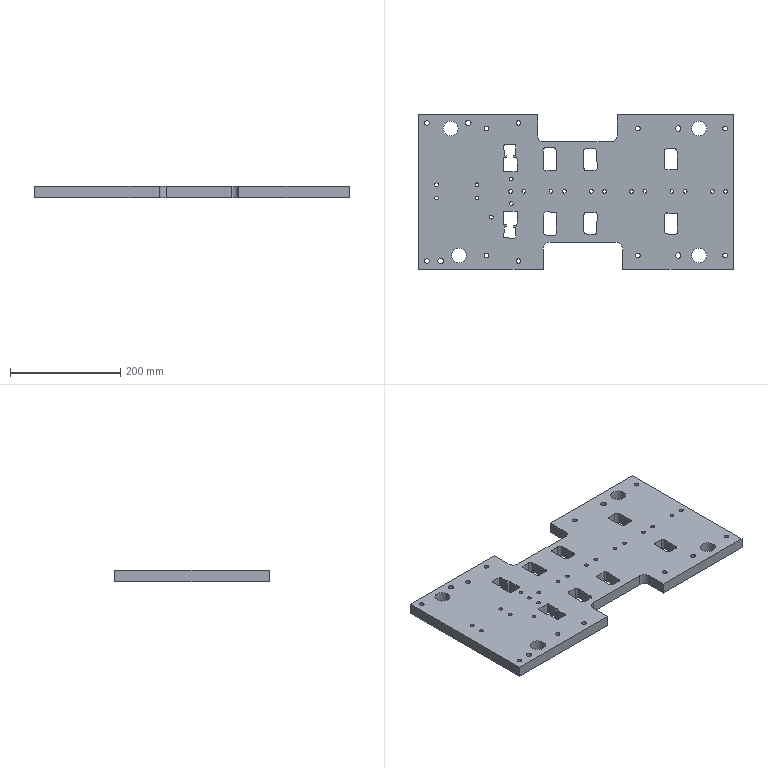Part | NX | features PPS-2 2 | 1 solid | 169 faces | box 570 x 280 x 20 mm | volume 2679314 mm3 | cylinder 94 | plane 62 | cone 13 | commonest cylinder face diameters 8 x21 4 x16 6.805 x16 10 x14 8.5 x10 12 x6